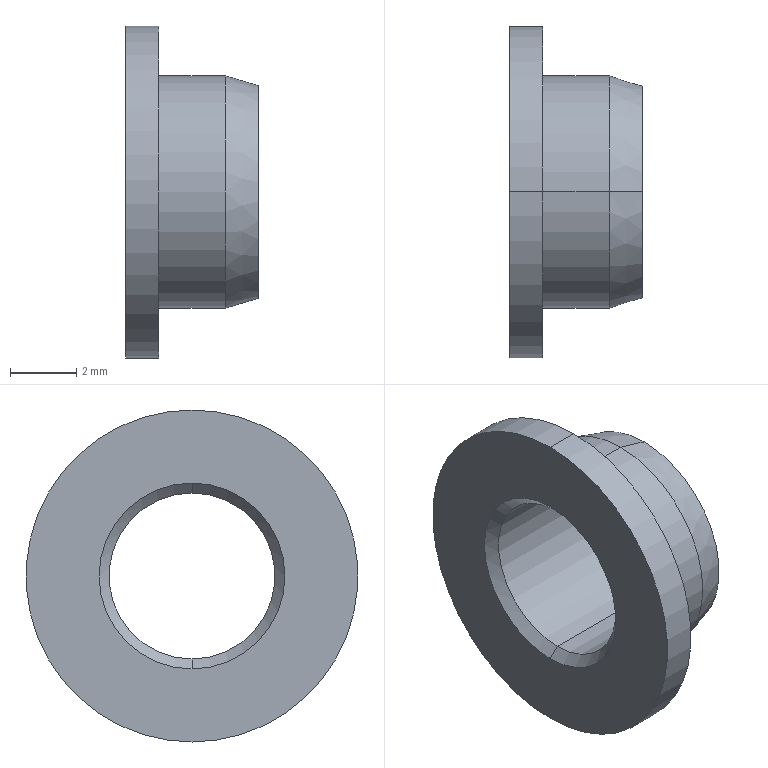Part | STEP file | 0246_010_JZF5-3 | 1 solid | 13 faces | box 4 x 10 x 10 mm | volume 111.514 mm3 | cylinder 6 | cone 4 | plane 3 | commonest cylinder face diameters 5 x2 7 x2 10 x2
STEP:
#1=CARTESIAN_POINT('',(0.,0.,0.));
#2=DIRECTION('',(0.,0.,1.));
#3=DIRECTION('',(1.,0.,0.));
#4=AXIS2_PLACEMENT_3D('',#1,#2,#3);
#5=CARTESIAN_POINT('',(0.,0.,5.));
#6=VERTEX_POINT('',#5);
#7=CARTESIAN_POINT('',(0.,0.,-5.));
#8=VERTEX_POINT('',#7);
#9=CARTESIAN_POINT('',(0.,0.,0.));
#10=DIRECTION('',(-1.,0.,0.));
#11=DIRECTION('',(0.,0.,-1.));
#12=AXIS2_PLACEMENT_3D('',#9,#10,#11);
#13=CIRCLE('',#12,5.);
#14=CARTESIAN_POINT('',(0.5,0.,0.));
#15=DIRECTION('',(1.,0.,0.));
#16=DIRECTION('',(0.,0.,-1.));
#17=AXIS2_PLACEMENT_3D('',#14,#15,#16);
#18=CYLINDRICAL_SURFACE('',#17,5.);
#19=CARTESIAN_POINT('',(6.283,-0.5));
#20=DIRECTION('',(-1.,0.));
#21=VECTOR('',#20,1.);
#22=LINE('',#19,#21);
#23=(GEOMETRIC_REPRESENTATION_CONTEXT(2)PARAMETRIC_REPRESENTATION_CONTEXT()REPRESENTATION_CONTEXT('',''));
#24=DEFINITIONAL_REPRESENTATION('',(#22),#23);
#25=PCURVE('',#18,#24);
#26=CARTESIAN_POINT('',(0.,3.9,0.));
#27=DIRECTION('',(-1.,0.,0.));
#28=DIRECTION('',(0.,0.,1.));
#29=AXIS2_PLACEMENT_3D('',#26,#27,#28);
#30=PLANE('',#29);
#31=CARTESIAN_POINT('',(0.,-3.9));
#32=DIRECTION('',(-1.,0.));
#33=AXIS2_PLACEMENT_2D('',#31,#32);
#34=CIRCLE('',#33,5.);
#35=(GEOMETRIC_REPRESENTATION_CONTEXT(2)PARAMETRIC_REPRESENTATION_CONTEXT()REPRESENTATION_CONTEXT('',''));
#36=DEFINITIONAL_REPRESENTATION('',(#34),#35);
#37=PCURVE('',#30,#36);
#38=SURFACE_CURVE('',#13,(#25,#37),.PCURVE_S1.);
#39=EDGE_CURVE('',#6,#8,#38,.T.);
#40=ORIENTED_EDGE('',*,*,#39,.F.);
#41=CARTESIAN_POINT('',(1.,0.,5.));
#42=VERTEX_POINT('',#41);
#43=CARTESIAN_POINT('',(0.5,0.,5.));
#44=DIRECTION('',(1.,0.,0.));
#45=VECTOR('',#44,1.);
#46=LINE('',#43,#45);
#47=CARTESIAN_POINT('',(3.142,0.));
#48=DIRECTION('',(0.,1.));
#49=VECTOR('',#48,1.);
#50=LINE('',#47,#49);
#51=(GEOMETRIC_REPRESENTATION_CONTEXT(2)PARAMETRIC_REPRESENTATION_CONTEXT()REPRESENTATION_CONTEXT('',''));
#52=DEFINITIONAL_REPRESENTATION('',(#50),#51);
#53=PCURVE('',#18,#52);
#54=CARTESIAN_POINT('',(0.5,0.,0.));
#55=DIRECTION('',(1.,0.,0.));
#56=DIRECTION('',(0.,0.,-1.));
#57=AXIS2_PLACEMENT_3D('',#54,#55,#56);
#58=CYLINDRICAL_SURFACE('',#57,5.);
#59=CARTESIAN_POINT('',(3.142,0.));
#60=DIRECTION('',(0.,1.));
#61=VECTOR('',#60,1.);
#62=LINE('',#59,#61);
#63=(GEOMETRIC_REPRESENTATION_CONTEXT(2)PARAMETRIC_REPRESENTATION_CONTEXT()REPRESENTATION_CONTEXT('',''));
#64=DEFINITIONAL_REPRESENTATION('',(#62),#63);
#65=PCURVE('',#58,#64);
#66=SURFACE_CURVE('',#46,(#53,#65),.PCURVE_S1.);
#67=EDGE_CURVE('',#6,#42,#66,.T.);
#68=ORIENTED_EDGE('',*,*,#67,.T.);
#69=CARTESIAN_POINT('',(1.,0.,-5.));
#70=VERTEX_POINT('',#69);
#71=CARTESIAN_POINT('',(1.,0.,0.));
#72=DIRECTION('',(-1.,0.,0.));
#73=DIRECTION('',(0.,0.,-1.));
#74=AXIS2_PLACEMENT_3D('',#71,#72,#73);
#75=CIRCLE('',#74,5.);
#76=CARTESIAN_POINT('',(6.283,0.5));
#77=DIRECTION('',(-1.,0.));
#78=VECTOR('',#77,1.);
#79=LINE('',#76,#78);
#80=(GEOMETRIC_REPRESENTATION_CONTEXT(2)PARAMETRIC_REPRESENTATION_CONTEXT()REPRESENTATION_CONTEXT('',''));
#81=DEFINITIONAL_REPRESENTATION('',(#79),#80);
#82=PCURVE('',#18,#81);
#83=CARTESIAN_POINT('',(1.,4.25,0.));
#84=DIRECTION('',(1.,0.,0.));
#85=DIRECTION('',(0.,0.,-1.));
#86=AXIS2_PLACEMENT_3D('',#83,#84,#85);
#87=PLANE('',#86);
#88=CARTESIAN_POINT('',(5.,-4.25));
#89=CARTESIAN_POINT('',(5.,-12.91));
#90=CARTESIAN_POINT('',(-2.5,-8.58));
#91=CARTESIAN_POINT('',(-10.,-4.25));
#92=CARTESIAN_POINT('',(-2.5,0.08013));
#93=CARTESIAN_POINT('',(5.,4.41));
#94=CARTESIAN_POINT('',(5.,-4.25));
#95=(BOUNDED_CURVE()B_SPLINE_CURVE(2,(#88,#89,#90,#91,#92,#93,#94),.UNSPECIFIED.,.T.,.F.)B_SPLINE_CURVE_WITH_KNOTS((1,2,2,2,2,1),(-2.094,0.,2.094,4.189,6.283,8.378),.UNSPECIFIED.)CURVE()GEOMETRIC_REPRESENTATION_ITEM()RATIONAL_B_SPLINE_CURVE((1.,0.5,1.,0.5,1.,0.5,1.))REPRESENTATION_ITEM(''));
#96=(GEOMETRIC_REPRESENTATION_CONTEXT(2)PARAMETRIC_REPRESENTATION_CONTEXT()REPRESENTATION_CONTEXT('',''));
#97=DEFINITIONAL_REPRESENTATION('',(#95),#96);
#98=PCURVE('',#87,#97);
#99=SURFACE_CURVE('',#75,(#82,#98),.PCURVE_S1.);
#100=EDGE_CURVE('',#42,#70,#99,.T.);
#101=ORIENTED_EDGE('',*,*,#100,.T.);
#102=CARTESIAN_POINT('',(0.5,0.,-5.));
#103=DIRECTION('',(1.,0.,0.));
#104=VECTOR('',#103,1.);
#105=LINE('',#102,#104);
#106=CARTESIAN_POINT('',(0.,0.));
#107=DIRECTION('',(0.,1.));
#108=VECTOR('',#107,1.);
#109=LINE('',#106,#108);
#110=(GEOMETRIC_REPRESENTATION_CONTEXT(2)PARAMETRIC_REPRESENTATION_CONTEXT()REPRESENTATION_CONTEXT('',''));
#111=DEFINITIONAL_REPRESENTATION('',(#109),#110);
#112=PCURVE('',#18,#111);
#113=CARTESIAN_POINT('',(6.283,0.));
#114=DIRECTION('',(0.,1.));
#115=VECTOR('',#114,1.);
#116=LINE('',#113,#115);
#117=(GEOMETRIC_REPRESENTATION_CONTEXT(2)PARAMETRIC_REPRESENTATION_CONTEXT()REPRESENTATION_CONTEXT('',''));
#118=DEFINITIONAL_REPRESENTATION('',(#116),#117);
#119=PCURVE('',#58,#118);
#120=SURFACE_CURVE('',#105,(#112,#119),.PCURVE_S1.);
#121=EDGE_CURVE('',#8,#70,#120,.T.);
#122=ORIENTED_EDGE('',*,*,#121,.F.);
#123=EDGE_LOOP('',(#40,#68,#101,#122));
#124=FACE_BOUND('',#123,.T.);
#125=ADVANCED_FACE('',(#124),#18,.T.);
#126=CARTESIAN_POINT('',(0.3,0.,2.5));
#127=VERTEX_POINT('',#126);
#128=CARTESIAN_POINT('',(0.,0.,2.8));
#129=VERTEX_POINT('',#128);
#130=CARTESIAN_POINT('',(0.,0.,2.8));
#131=DIRECTION('',(-0.7071,0.,0.7071));
#132=VECTOR('',#131,1.);
#133=LINE('',#130,#132);
#134=CARTESIAN_POINT('',(0.,0.,0.));
#135=DIRECTION('',(-1.,0.,0.));
#136=DIRECTION('',(0.,0.,1.));
#137=AXIS2_PLACEMENT_3D('',#134,#135,#136);
#138=CONICAL_SURFACE('',#137,2.8,0.7854);
#139=CARTESIAN_POINT('',(6.283,0.));
#140=DIRECTION('',(0.,1.));
#141=VECTOR('',#140,1.);
#142=LINE('',#139,#141);
#143=(GEOMETRIC_REPRESENTATION_CONTEXT(2)PARAMETRIC_REPRESENTATION_CONTEXT()REPRESENTATION_CONTEXT('',''));
#144=DEFINITIONAL_REPRESENTATION('',(#142),#143);
#145=PCURVE('',#138,#144);
#146=CARTESIAN_POINT('',(0.,0.,0.));
#147=DIRECTION('',(-1.,0.,0.));
#148=DIRECTION('',(0.,0.,1.));
#149=AXIS2_PLACEMENT_3D('',#146,#147,#148);
#150=CONICAL_SURFACE('',#149,2.8,0.7854);
#151=CARTESIAN_POINT('',(0.,0.));
#152=DIRECTION('',(0.,1.));
#153=VECTOR('',#152,1.);
#154=LINE('',#151,#153);
#155=(GEOMETRIC_REPRESENTATION_CONTEXT(2)PARAMETRIC_REPRESENTATION_CONTEXT()REPRESENTATION_CONTEXT('',''));
#156=DEFINITIONAL_REPRESENTATION('',(#154),#155);
#157=PCURVE('',#150,#156);
#158=SURFACE_CURVE('',#133,(#145,#157),.PCURVE_S1.);
#159=EDGE_CURVE('',#127,#129,#158,.T.);
#160=ORIENTED_EDGE('',*,*,#159,.T.);
#161=CARTESIAN_POINT('',(0.,0.,-2.8));
#162=VERTEX_POINT('',#161);
#163=CARTESIAN_POINT('',(0.,0.,0.));
#164=DIRECTION('',(1.,0.,0.));
#165=DIRECTION('',(0.,0.,1.));
#166=AXIS2_PLACEMENT_3D('',#163,#164,#165);
#167=CIRCLE('',#166,2.8);
#168=CARTESIAN_POINT('',(6.283,0.));
#169=DIRECTION('',(-1.,0.));
#170=VECTOR('',#169,1.);
#171=LINE('',#168,#170);
#172=(GEOMETRIC_REPRESENTATION_CONTEXT(2)PARAMETRIC_REPRESENTATION_CONTEXT()REPRESENTATION_CONTEXT('',''));
#173=DEFINITIONAL_REPRESENTATION('',(#171),#172);
#174=PCURVE('',#138,#173);
#175=CARTESIAN_POINT('',(2.8,-3.9));
#176=CARTESIAN_POINT('',(2.8,-8.75));
#177=CARTESIAN_POINT('',(-1.4,-6.325));
#178=CARTESIAN_POINT('',(-5.6,-3.9));
#179=CARTESIAN_POINT('',(-1.4,-1.475));
#180=CARTESIAN_POINT('',(2.8,0.9497));
#181=CARTESIAN_POINT('',(2.8,-3.9));
#182=(BOUNDED_CURVE()B_SPLINE_CURVE(2,(#175,#176,#177,#178,#179,#180,#181),.UNSPECIFIED.,.T.,.F.)B_SPLINE_CURVE_WITH_KNOTS((1,2,2,2,2,1),(-2.094,0.,2.094,4.189,6.283,8.378),.UNSPECIFIED.)CURVE()GEOMETRIC_REPRESENTATION_ITEM()RATIONAL_B_SPLINE_CURVE((1.,0.5,1.,0.5,1.,0.5,1.))REPRESENTATION_ITEM(''));
#183=(GEOMETRIC_REPRESENTATION_CONTEXT(2)PARAMETRIC_REPRESENTATION_CONTEXT()REPRESENTATION_CONTEXT('',''));
#184=DEFINITIONAL_REPRESENTATION('',(#182),#183);
#185=PCURVE('',#30,#184);
#186=SURFACE_CURVE('',#167,(#174,#185),.PCURVE_S1.);
#187=EDGE_CURVE('',#129,#162,#186,.T.);
#188=ORIENTED_EDGE('',*,*,#187,.T.);
#189=CARTESIAN_POINT('',(0.3,0.,-2.5));
#190=VERTEX_POINT('',#189);
#191=CARTESIAN_POINT('',(0.,0.,-2.8));
#192=DIRECTION('',(-0.7071,0.,-0.7071));
#193=VECTOR('',#192,1.);
#194=LINE('',#191,#193);
#195=CARTESIAN_POINT('',(3.142,0.));
#196=DIRECTION('',(0.,1.));
#197=VECTOR('',#196,1.);
#198=LINE('',#195,#197);
#199=(GEOMETRIC_REPRESENTATION_CONTEXT(2)PARAMETRIC_REPRESENTATION_CONTEXT()REPRESENTATION_CONTEXT('',''));
#200=DEFINITIONAL_REPRESENTATION('',(#198),#199);
#201=PCURVE('',#138,#200);
#202=CARTESIAN_POINT('',(3.142,0.));
#203=DIRECTION('',(0.,1.));
#204=VECTOR('',#203,1.);
#205=LINE('',#202,#204);
#206=(GEOMETRIC_REPRESENTATION_CONTEXT(2)PARAMETRIC_REPRESENTATION_CONTEXT()REPRESENTATION_CONTEXT('',''));
#207=DEFINITIONAL_REPRESENTATION('',(#205),#206);
#208=PCURVE('',#150,#207);
#209=SURFACE_CURVE('',#194,(#201,#208),.PCURVE_S1.);
#210=EDGE_CURVE('',#190,#162,#209,.T.);
#211=ORIENTED_EDGE('',*,*,#210,.F.);
#212=CARTESIAN_POINT('',(0.3,0.,0.));
#213=DIRECTION('',(-1.,0.,0.));
#214=DIRECTION('',(0.,1.,0.));
#215=AXIS2_PLACEMENT_3D('',#212,#213,#214);
#216=CIRCLE('',#215,2.5);
#217=CARTESIAN_POINT('',(1.571,-0.3));
#218=DIRECTION('',(1.,0.));
#219=VECTOR('',#218,1.);
#220=LINE('',#217,#219);
#221=(GEOMETRIC_REPRESENTATION_CONTEXT(2)PARAMETRIC_REPRESENTATION_CONTEXT()REPRESENTATION_CONTEXT('',''));
#222=DEFINITIONAL_REPRESENTATION('',(#220),#221);
#223=PCURVE('',#138,#222);
#224=CARTESIAN_POINT('',(2.15,0.,0.));
#225=DIRECTION('',(1.,0.,0.));
#226=DIRECTION('',(0.,0.,-1.));
#227=AXIS2_PLACEMENT_3D('',#224,#225,#226);
#228=CYLINDRICAL_SURFACE('',#227,2.5);
#229=CARTESIAN_POINT('',(7.854,-1.85));
#230=DIRECTION('',(-1.,0.));
#231=VECTOR('',#230,1.);
#232=LINE('',#229,#231);
#233=(GEOMETRIC_REPRESENTATION_CONTEXT(2)PARAMETRIC_REPRESENTATION_CONTEXT()REPRESENTATION_CONTEXT('',''));
#234=DEFINITIONAL_REPRESENTATION('',(#232),#233);
#235=PCURVE('',#228,#234);
#236=SURFACE_CURVE('',#216,(#223,#235),.PCURVE_S1.);
#237=EDGE_CURVE('',#190,#127,#236,.T.);
#238=ORIENTED_EDGE('',*,*,#237,.T.);
#239=EDGE_LOOP('',(#160,#188,#211,#238));
#240=FACE_BOUND('',#239,.F.);
#241=ADVANCED_FACE('',(#240),#138,.F.);
#242=CARTESIAN_POINT('',(4.,0.,-2.5));
#243=VERTEX_POINT('',#242);
#244=CARTESIAN_POINT('',(2.15,0.,-2.5));
#245=DIRECTION('',(1.,0.,0.));
#246=VECTOR('',#245,1.);
#247=LINE('',#244,#246);
#248=CARTESIAN_POINT('',(6.283,0.));
#249=DIRECTION('',(0.,1.));
#250=VECTOR('',#249,1.);
#251=LINE('',#248,#250);
#252=(GEOMETRIC_REPRESENTATION_CONTEXT(2)PARAMETRIC_REPRESENTATION_CONTEXT()REPRESENTATION_CONTEXT('',''));
#253=DEFINITIONAL_REPRESENTATION('',(#251),#252);
#254=PCURVE('',#228,#253);
#255=CARTESIAN_POINT('',(2.15,0.,0.));
#256=DIRECTION('',(1.,0.,0.));
#257=DIRECTION('',(0.,0.,-1.));
#258=AXIS2_PLACEMENT_3D('',#255,#256,#257);
#259=CYLINDRICAL_SURFACE('',#258,2.5);
#260=CARTESIAN_POINT('',(0.,0.));
#261=DIRECTION('',(0.,1.));
#262=VECTOR('',#261,1.);
#263=LINE('',#260,#262);
#264=(GEOMETRIC_REPRESENTATION_CONTEXT(2)PARAMETRIC_REPRESENTATION_CONTEXT()REPRESENTATION_CONTEXT('',''));
#265=DEFINITIONAL_REPRESENTATION('',(#263),#264);
#266=PCURVE('',#259,#265);
#267=SURFACE_CURVE('',#247,(#254,#266),.PCURVE_S1.);
#268=EDGE_CURVE('',#190,#243,#267,.T.);
#269=ORIENTED_EDGE('',*,*,#268,.T.);
#270=CARTESIAN_POINT('',(4.,0.,2.5));
#271=VERTEX_POINT('',#270);
#272=CARTESIAN_POINT('',(4.,0.,0.));
#273=DIRECTION('',(-1.,0.,0.));
#274=DIRECTION('',(0.,0.,-1.));
#275=AXIS2_PLACEMENT_3D('',#272,#273,#274);
#276=CIRCLE('',#275,2.5);
#277=CARTESIAN_POINT('',(6.283,1.85));
#278=DIRECTION('',(-1.,0.));
#279=VECTOR('',#278,1.);
#280=LINE('',#277,#279);
#281=(GEOMETRIC_REPRESENTATION_CONTEXT(2)PARAMETRIC_REPRESENTATION_CONTEXT()REPRESENTATION_CONTEXT('',''));
#282=DEFINITIONAL_REPRESENTATION('',(#280),#281);
#283=PCURVE('',#228,#282);
#284=CARTESIAN_POINT('',(4.,2.85,0.));
#285=DIRECTION('',(1.,0.,0.));
#286=DIRECTION('',(0.,0.,-1.));
#287=AXIS2_PLACEMENT_3D('',#284,#285,#286);
#288=PLANE('',#287);
#289=CARTESIAN_POINT('',(2.5,-2.85));
#290=CARTESIAN_POINT('',(2.5,-7.18));
#291=CARTESIAN_POINT('',(-1.25,-5.015));
#292=CARTESIAN_POINT('',(-5.,-2.85));
#293=CARTESIAN_POINT('',(-1.25,-0.6849));
#294=CARTESIAN_POINT('',(2.5,1.48));
#295=CARTESIAN_POINT('',(2.5,-2.85));
#296=(BOUNDED_CURVE()B_SPLINE_CURVE(2,(#289,#290,#291,#292,#293,#294,#295),.UNSPECIFIED.,.T.,.F.)B_SPLINE_CURVE_WITH_KNOTS((1,2,2,2,2,1),(-2.094,0.,2.094,4.189,6.283,8.378),.UNSPECIFIED.)CURVE()GEOMETRIC_REPRESENTATION_ITEM()RATIONAL_B_SPLINE_CURVE((1.,0.5,1.,0.5,1.,0.5,1.))REPRESENTATION_ITEM(''));
#297=(GEOMETRIC_REPRESENTATION_CONTEXT(2)PARAMETRIC_REPRESENTATION_CONTEXT()REPRESENTATION_CONTEXT('',''));
#298=DEFINITIONAL_REPRESENTATION('',(#296),#297);
#299=PCURVE('',#288,#298);
#300=SURFACE_CURVE('',#276,(#283,#299),.PCURVE_S1.);
#301=EDGE_CURVE('',#243,#271,#300,.T.);
#302=ORIENTED_EDGE('',*,*,#301,.T.);
#303=CARTESIAN_POINT('',(2.15,0.,2.5));
#304=DIRECTION('',(1.,0.,0.));
#305=VECTOR('',#304,1.);
#306=LINE('',#303,#305);
#307=CARTESIAN_POINT('',(3.142,0.));
#308=DIRECTION('',(0.,1.));
#309=VECTOR('',#308,1.);
#310=LINE('',#307,#309);
#311=(GEOMETRIC_REPRESENTATION_CONTEXT(2)PARAMETRIC_REPRESENTATION_CONTEXT()REPRESENTATION_CONTEXT('',''));
#312=DEFINITIONAL_REPRESENTATION('',(#310),#311);
#313=PCURVE('',#228,#312);
#314=CARTESIAN_POINT('',(3.142,0.));
#315=DIRECTION('',(0.,1.));
#316=VECTOR('',#315,1.);
#317=LINE('',#314,#316);
#318=(GEOMETRIC_REPRESENTATION_CONTEXT(2)PARAMETRIC_REPRESENTATION_CONTEXT()REPRESENTATION_CONTEXT('',''));
#319=DEFINITIONAL_REPRESENTATION('',(#317),#318);
#320=PCURVE('',#259,#319);
#321=SURFACE_CURVE('',#306,(#313,#320),.PCURVE_S1.);
#322=EDGE_CURVE('',#127,#271,#321,.T.);
#323=ORIENTED_EDGE('',*,*,#322,.F.);
#324=ORIENTED_EDGE('',*,*,#237,.F.);
#325=EDGE_LOOP('',(#269,#302,#323,#324));
#326=FACE_BOUND('',#325,.F.);
#327=ADVANCED_FACE('',(#326),#228,.F.);
#328=CARTESIAN_POINT('',(1.,0.,3.5));
#329=VERTEX_POINT('',#328);
#330=CARTESIAN_POINT('',(1.,0.,-3.5));
#331=VERTEX_POINT('',#330);
#332=CARTESIAN_POINT('',(1.,0.,0.));
#333=DIRECTION('',(-1.,0.,0.));
#334=DIRECTION('',(0.,0.,-1.));
#335=AXIS2_PLACEMENT_3D('',#332,#333,#334);
#336=CIRCLE('',#335,3.5);
#337=CARTESIAN_POINT('',(2.,0.,0.));
#338=DIRECTION('',(1.,0.,0.));
#339=DIRECTION('',(0.,0.,-1.));
#340=AXIS2_PLACEMENT_3D('',#337,#338,#339);
#341=CYLINDRICAL_SURFACE('',#340,3.5);
#342=CARTESIAN_POINT('',(6.283,-1.));
#343=DIRECTION('',(-1.,0.));
#344=VECTOR('',#343,1.);
#345=LINE('',#342,#344);
#346=(GEOMETRIC_REPRESENTATION_CONTEXT(2)PARAMETRIC_REPRESENTATION_CONTEXT()REPRESENTATION_CONTEXT('',''));
#347=DEFINITIONAL_REPRESENTATION('',(#345),#346);
#348=PCURVE('',#341,#347);
#349=CARTESIAN_POINT('',(3.5,-4.25));
#350=CARTESIAN_POINT('',(3.5,-10.312));
#351=CARTESIAN_POINT('',(-1.75,-7.281));
#352=CARTESIAN_POINT('',(-7.,-4.25));
#353=CARTESIAN_POINT('',(-1.75,-1.219));
#354=CARTESIAN_POINT('',(3.5,1.812));
#355=CARTESIAN_POINT('',(3.5,-4.25));
#356=(BOUNDED_CURVE()B_SPLINE_CURVE(2,(#349,#350,#351,#352,#353,#354,#355),.UNSPECIFIED.,.T.,.F.)B_SPLINE_CURVE_WITH_KNOTS((1,2,2,2,2,1),(-2.094,0.,2.094,4.189,6.283,8.378),.UNSPECIFIED.)CURVE()GEOMETRIC_REPRESENTATION_ITEM()RATIONAL_B_SPLINE_CURVE((1.,0.5,1.,0.5,1.,0.5,1.))REPRESENTATION_ITEM(''));
#357=(GEOMETRIC_REPRESENTATION_CONTEXT(2)PARAMETRIC_REPRESENTATION_CONTEXT()REPRESENTATION_CONTEXT('',''));
#358=DEFINITIONAL_REPRESENTATION('',(#356),#357);
#359=PCURVE('',#87,#358);
#360=SURFACE_CURVE('',#336,(#348,#359),.PCURVE_S1.);
#361=EDGE_CURVE('',#329,#331,#360,.T.);
#362=ORIENTED_EDGE('',*,*,#361,.F.);
#363=CARTESIAN_POINT('',(3.,0.,3.5));
#364=VERTEX_POINT('',#363);
#365=CARTESIAN_POINT('',(2.,0.,3.5));
#366=DIRECTION('',(1.,0.,0.));
#367=VECTOR('',#366,1.);
#368=LINE('',#365,#367);
#369=CARTESIAN_POINT('',(3.142,0.));
#370=DIRECTION('',(0.,1.));
#371=VECTOR('',#370,1.);
#372=LINE('',#369,#371);
#373=(GEOMETRIC_REPRESENTATION_CONTEXT(2)PARAMETRIC_REPRESENTATION_CONTEXT()REPRESENTATION_CONTEXT('',''));
#374=DEFINITIONAL_REPRESENTATION('',(#372),#373);
#375=PCURVE('',#341,#374);
#376=CARTESIAN_POINT('',(2.,0.,0.));
#377=DIRECTION('',(1.,0.,0.));
#378=DIRECTION('',(0.,0.,-1.));
#379=AXIS2_PLACEMENT_3D('',#376,#377,#378);
#380=CYLINDRICAL_SURFACE('',#379,3.5);
#381=CARTESIAN_POINT('',(3.142,0.));
#382=DIRECTION('',(0.,1.));
#383=VECTOR('',#382,1.);
#384=LINE('',#381,#383);
#385=(GEOMETRIC_REPRESENTATION_CONTEXT(2)PARAMETRIC_REPRESENTATION_CONTEXT()REPRESENTATION_CONTEXT('',''));
#386=DEFINITIONAL_REPRESENTATION('',(#384),#385);
#387=PCURVE('',#380,#386);
#388=SURFACE_CURVE('',#368,(#375,#387),.PCURVE_S1.);
#389=EDGE_CURVE('',#329,#364,#388,.T.);
#390=ORIENTED_EDGE('',*,*,#389,.T.);
#391=CARTESIAN_POINT('',(3.,0.,-3.5));
#392=VERTEX_POINT('',#391);
#393=CARTESIAN_POINT('',(3.,0.,0.));
#394=DIRECTION('',(-1.,0.,0.));
#395=DIRECTION('',(0.,0.,-1.));
#396=AXIS2_PLACEMENT_3D('',#393,#394,#395);
#397=CIRCLE('',#396,3.5);
#398=CARTESIAN_POINT('',(6.283,1.));
#399=DIRECTION('',(-1.,0.));
#400=VECTOR('',#399,1.);
#401=LINE('',#398,#400);
#402=(GEOMETRIC_REPRESENTATION_CONTEXT(2)PARAMETRIC_REPRESENTATION_CONTEXT()REPRESENTATION_CONTEXT('',''));
#403=DEFINITIONAL_REPRESENTATION('',(#401),#402);
#404=PCURVE('',#341,#403);
#405=CARTESIAN_POINT('',(3.,0.,0.));
#406=DIRECTION('',(-1.,0.,0.));
#407=DIRECTION('',(0.,0.,1.));
#408=AXIS2_PLACEMENT_3D('',#405,#406,#407);
#409=CONICAL_SURFACE('',#408,3.5,0.2915);
#410=CARTESIAN_POINT('',(-3.142,0.));
#411=DIRECTION('',(1.,0.));
#412=VECTOR('',#411,1.);
#413=LINE('',#410,#412);
#414=(GEOMETRIC_REPRESENTATION_CONTEXT(2)PARAMETRIC_REPRESENTATION_CONTEXT()REPRESENTATION_CONTEXT('',''));
#415=DEFINITIONAL_REPRESENTATION('',(#413),#414);
#416=PCURVE('',#409,#415);
#417=SURFACE_CURVE('',#397,(#404,#416),.PCURVE_S1.);
#418=EDGE_CURVE('',#364,#392,#417,.T.);
#419=ORIENTED_EDGE('',*,*,#418,.T.);
#420=CARTESIAN_POINT('',(2.,0.,-3.5));
#421=DIRECTION('',(1.,0.,0.));
#422=VECTOR('',#421,1.);
#423=LINE('',#420,#422);
#424=CARTESIAN_POINT('',(0.,0.));
#425=DIRECTION('',(0.,1.));
#426=VECTOR('',#425,1.);
#427=LINE('',#424,#426);
#428=(GEOMETRIC_REPRESENTATION_CONTEXT(2)PARAMETRIC_REPRESENTATION_CONTEXT()REPRESENTATION_CONTEXT('',''));
#429=DEFINITIONAL_REPRESENTATION('',(#427),#428);
#430=PCURVE('',#341,#429);
#431=CARTESIAN_POINT('',(6.283,0.));
#432=DIRECTION('',(0.,1.));
#433=VECTOR('',#432,1.);
#434=LINE('',#431,#433);
#435=(GEOMETRIC_REPRESENTATION_CONTEXT(2)PARAMETRIC_REPRESENTATION_CONTEXT()REPRESENTATION_CONTEXT('',''));
#436=DEFINITIONAL_REPRESENTATION('',(#434),#435);
#437=PCURVE('',#380,#436);
#438=SURFACE_CURVE('',#423,(#430,#437),.PCURVE_S1.);
#439=EDGE_CURVE('',#331,#392,#438,.T.);
#440=ORIENTED_EDGE('',*,*,#439,.F.);
#441=EDGE_LOOP('',(#362,#390,#419,#440));
#442=FACE_BOUND('',#441,.T.);
#443=ADVANCED_FACE('',(#442),#341,.T.);
#444=CARTESIAN_POINT('',(4.,0.,-3.2));
#445=VERTEX_POINT('',#444);
#446=CARTESIAN_POINT('',(4.,0.,3.2));
#447=VERTEX_POINT('',#446);
#448=CARTESIAN_POINT('',(4.,0.,0.));
#449=DIRECTION('',(1.,0.,0.));
#450=DIRECTION('',(0.,0.,1.));
#451=AXIS2_PLACEMENT_3D('',#448,#449,#450);
#452=CIRCLE('',#451,3.2);
#453=CARTESIAN_POINT('',(6.283,-1.));
#454=DIRECTION('',(-1.,0.));
#455=VECTOR('',#454,1.);
#456=LINE('',#453,#455);
#457=(GEOMETRIC_REPRESENTATION_CONTEXT(2)PARAMETRIC_REPRESENTATION_CONTEXT()REPRESENTATION_CONTEXT('',''));
#458=DEFINITIONAL_REPRESENTATION('',(#456),#457);
#459=PCURVE('',#409,#458);
#460=CARTESIAN_POINT('',(0.,-2.85));
#461=DIRECTION('',(-1.,0.));
#462=AXIS2_PLACEMENT_2D('',#460,#461);
#463=CIRCLE('',#462,3.2);
#464=(GEOMETRIC_REPRESENTATION_CONTEXT(2)PARAMETRIC_REPRESENTATION_CONTEXT()REPRESENTATION_CONTEXT('',''));
#465=DEFINITIONAL_REPRESENTATION('',(#463),#464);
#466=PCURVE('',#288,#465);
#467=SURFACE_CURVE('',#452,(#459,#466),.PCURVE_S1.);
#468=EDGE_CURVE('',#445,#447,#467,.T.);
#469=ORIENTED_EDGE('',*,*,#468,.F.);
#470=CARTESIAN_POINT('',(3.,0.,-3.5));
#471=DIRECTION('',(-0.9578,0.,-0.2873));
#472=VECTOR('',#471,1.);
#473=LINE('',#470,#472);
#474=CARTESIAN_POINT('',(3.142,0.));
#475=DIRECTION('',(0.,1.));
#476=VECTOR('',#475,1.);
#477=LINE('',#474,#476);
#478=(GEOMETRIC_REPRESENTATION_CONTEXT(2)PARAMETRIC_REPRESENTATION_CONTEXT()REPRESENTATION_CONTEXT('',''));
#479=DEFINITIONAL_REPRESENTATION('',(#477),#478);
#480=PCURVE('',#409,#479);
#481=CARTESIAN_POINT('',(3.,0.,0.));
#482=DIRECTION('',(-1.,0.,0.));
#483=DIRECTION('',(0.,0.,1.));
#484=AXIS2_PLACEMENT_3D('',#481,#482,#483);
#485=CONICAL_SURFACE('',#484,3.5,0.2915);
#486=CARTESIAN_POINT('',(3.142,0.));
#487=DIRECTION('',(0.,1.));
#488=VECTOR('',#487,1.);
#489=LINE('',#486,#488);
#490=(GEOMETRIC_REPRESENTATION_CONTEXT(2)PARAMETRIC_REPRESENTATION_CONTEXT()REPRESENTATION_CONTEXT('',''));
#491=DEFINITIONAL_REPRESENTATION('',(#489),#490);
#492=PCURVE('',#485,#491);
#493=SURFACE_CURVE('',#473,(#480,#492),.PCURVE_S1.);
#494=EDGE_CURVE('',#445,#392,#493,.T.);
#495=ORIENTED_EDGE('',*,*,#494,.T.);
#496=ORIENTED_EDGE('',*,*,#418,.F.);
#497=CARTESIAN_POINT('',(3.,0.,3.5));
#498=DIRECTION('',(-0.9578,0.,0.2873));
#499=VECTOR('',#498,1.);
#500=LINE('',#497,#499);
#501=CARTESIAN_POINT('',(0.,0.));
#502=DIRECTION('',(0.,1.));
#503=VECTOR('',#502,1.);
#504=LINE('',#501,#503);
#505=(GEOMETRIC_REPRESENTATION_CONTEXT(2)PARAMETRIC_REPRESENTATION_CONTEXT()REPRESENTATION_CONTEXT('',''));
#506=DEFINITIONAL_REPRESENTATION('',(#504),#505);
#507=PCURVE('',#409,#506);
#508=CARTESIAN_POINT('',(6.283,0.));
#509=DIRECTION('',(0.,1.));
#510=VECTOR('',#509,1.);
#511=LINE('',#508,#510);
#512=(GEOMETRIC_REPRESENTATION_CONTEXT(2)PARAMETRIC_REPRESENTATION_CONTEXT()REPRESENTATION_CONTEXT('',''));
#513=DEFINITIONAL_REPRESENTATION('',(#511),#512);
#514=PCURVE('',#485,#513);
#515=SURFACE_CURVE('',#500,(#507,#514),.PCURVE_S1.);
#516=EDGE_CURVE('',#447,#364,#515,.T.);
#517=ORIENTED_EDGE('',*,*,#516,.F.);
#518=EDGE_LOOP('',(#469,#495,#496,#517));
#519=FACE_BOUND('',#518,.T.);
#520=ADVANCED_FACE('',(#519),#409,.T.);
#521=CARTESIAN_POINT('',(0.,0.,0.));
#522=DIRECTION('',(-1.,0.,0.));
#523=DIRECTION('',(0.,0.,-1.));
#524=AXIS2_PLACEMENT_3D('',#521,#522,#523);
#525=CIRCLE('',#524,5.);
#526=CARTESIAN_POINT('',(0.,-3.9));
#527=DIRECTION('',(-1.,0.));
#528=AXIS2_PLACEMENT_2D('',#526,#527);
#529=CIRCLE('',#528,5.);
#530=(GEOMETRIC_REPRESENTATION_CONTEXT(2)PARAMETRIC_REPRESENTATION_CONTEXT()REPRESENTATION_CONTEXT('',''));
#531=DEFINITIONAL_REPRESENTATION('',(#529),#530);
#532=PCURVE('',#30,#531);
#533=CARTESIAN_POINT('',(6.283,-0.5));
#534=DIRECTION('',(-1.,0.));
#535=VECTOR('',#534,1.);
#536=LINE('',#533,#535);
#537=(GEOMETRIC_REPRESENTATION_CONTEXT(2)PARAMETRIC_REPRESENTATION_CONTEXT()REPRESENTATION_CONTEXT('',''));
#538=DEFINITIONAL_REPRESENTATION('',(#536),#537);
#539=PCURVE('',#58,#538);
#540=SURFACE_CURVE('',#525,(#532,#539),.PCURVE_S1.);
#541=EDGE_CURVE('',#8,#6,#540,.T.);
#542=ORIENTED_EDGE('',*,*,#541,.T.);
#543=ORIENTED_EDGE('',*,*,#39,.T.);
#544=EDGE_LOOP('',(#542,#543));
#545=FACE_BOUND('',#544,.T.);
#546=ORIENTED_EDGE('',*,*,#187,.T.);
#547=CARTESIAN_POINT('',(0.,0.,0.));
#548=DIRECTION('',(1.,0.,0.));
#549=DIRECTION('',(0.,0.,1.));
#550=AXIS2_PLACEMENT_3D('',#547,#548,#549);
#551=CIRCLE('',#550,2.8);
#552=CARTESIAN_POINT('',(2.8,-3.9));
#553=CARTESIAN_POINT('',(2.8,-8.75));
#554=CARTESIAN_POINT('',(-1.4,-6.325));
#555=CARTESIAN_POINT('',(-5.6,-3.9));
#556=CARTESIAN_POINT('',(-1.4,-1.475));
#557=CARTESIAN_POINT('',(2.8,0.9497));
#558=CARTESIAN_POINT('',(2.8,-3.9));
#559=(BOUNDED_CURVE()B_SPLINE_CURVE(2,(#552,#553,#554,#555,#556,#557,#558),.UNSPECIFIED.,.T.,.F.)B_SPLINE_CURVE_WITH_KNOTS((1,2,2,2,2,1),(-2.094,0.,2.094,4.189,6.283,8.378),.UNSPECIFIED.)CURVE()GEOMETRIC_REPRESENTATION_ITEM()RATIONAL_B_SPLINE_CURVE((1.,0.5,1.,0.5,1.,0.5,1.))REPRESENTATION_ITEM(''));
#560=(GEOMETRIC_REPRESENTATION_CONTEXT(2)PARAMETRIC_REPRESENTATION_CONTEXT()REPRESENTATION_CONTEXT('',''));
#561=DEFINITIONAL_REPRESENTATION('',(#559),#560);
#562=PCURVE('',#30,#561);
#563=CARTESIAN_POINT('',(6.283,0.));
#564=DIRECTION('',(-1.,0.));
#565=VECTOR('',#564,1.);
#566=LINE('',#563,#565);
#567=(GEOMETRIC_REPRESENTATION_CONTEXT(2)PARAMETRIC_REPRESENTATION_CONTEXT()REPRESENTATION_CONTEXT('',''));
#568=DEFINITIONAL_REPRESENTATION('',(#566),#567);
#569=PCURVE('',#150,#568);
#570=SURFACE_CURVE('',#551,(#562,#569),.PCURVE_S1.);
#571=EDGE_CURVE('',#162,#129,#570,.T.);
#572=ORIENTED_EDGE('',*,*,#571,.T.);
#573=EDGE_LOOP('',(#546,#572));
#574=FACE_BOUND('',#573,.T.);
#575=ADVANCED_FACE('',(#545,#574),#30,.T.);
#576=ORIENTED_EDGE('',*,*,#67,.F.);
#577=ORIENTED_EDGE('',*,*,#541,.F.);
#578=ORIENTED_EDGE('',*,*,#121,.T.);
#579=CARTESIAN_POINT('',(1.,0.,0.));
#580=DIRECTION('',(-1.,0.,0.));
#581=DIRECTION('',(0.,0.,-1.));
#582=AXIS2_PLACEMENT_3D('',#579,#580,#581);
#583=CIRCLE('',#582,5.);
#584=CARTESIAN_POINT('',(6.283,0.5));
#585=DIRECTION('',(-1.,0.));
#586=VECTOR('',#585,1.);
#587=LINE('',#584,#586);
#588=(GEOMETRIC_REPRESENTATION_CONTEXT(2)PARAMETRIC_REPRESENTATION_CONTEXT()REPRESENTATION_CONTEXT('',''));
#589=DEFINITIONAL_REPRESENTATION('',(#587),#588);
#590=PCURVE('',#58,#589);
#591=CARTESIAN_POINT('',(5.,-4.25));
#592=CARTESIAN_POINT('',(5.,-12.91));
#593=CARTESIAN_POINT('',(-2.5,-8.58));
#594=CARTESIAN_POINT('',(-10.,-4.25));
#595=CARTESIAN_POINT('',(-2.5,0.08013));
#596=CARTESIAN_POINT('',(5.,4.41));
#597=CARTESIAN_POINT('',(5.,-4.25));
#598=(BOUNDED_CURVE()B_SPLINE_CURVE(2,(#591,#592,#593,#594,#595,#596,#597),.UNSPECIFIED.,.T.,.F.)B_SPLINE_CURVE_WITH_KNOTS((1,2,2,2,2,1),(-2.094,0.,2.094,4.189,6.283,8.378),.UNSPECIFIED.)CURVE()GEOMETRIC_REPRESENTATION_ITEM()RATIONAL_B_SPLINE_CURVE((1.,0.5,1.,0.5,1.,0.5,1.))REPRESENTATION_ITEM(''));
#599=(GEOMETRIC_REPRESENTATION_CONTEXT(2)PARAMETRIC_REPRESENTATION_CONTEXT()REPRESENTATION_CONTEXT('',''));
#600=DEFINITIONAL_REPRESENTATION('',(#598),#599);
#601=PCURVE('',#87,#600);
#602=SURFACE_CURVE('',#583,(#590,#601),.PCURVE_S1.);
#603=EDGE_CURVE('',#70,#42,#602,.T.);
#604=ORIENTED_EDGE('',*,*,#603,.T.);
#605=EDGE_LOOP('',(#576,#577,#578,#604));
#606=FACE_BOUND('',#605,.T.);
#607=ADVANCED_FACE('',(#606),#58,.T.);
#608=ORIENTED_EDGE('',*,*,#571,.T.);
#609=ORIENTED_EDGE('',*,*,#159,.F.);
#610=CARTESIAN_POINT('',(0.3,0.,0.));
#611=DIRECTION('',(-1.,0.,0.));
#612=DIRECTION('',(0.,1.,0.));
#613=AXIS2_PLACEMENT_3D('',#610,#611,#612);
#614=CIRCLE('',#613,2.5);
#615=CARTESIAN_POINT('',(-4.712,-0.3));
#616=DIRECTION('',(1.,0.));
#617=VECTOR('',#616,1.);
#618=LINE('',#615,#617);
#619=(GEOMETRIC_REPRESENTATION_CONTEXT(2)PARAMETRIC_REPRESENTATION_CONTEXT()REPRESENTATION_CONTEXT('',''));
#620=DEFINITIONAL_REPRESENTATION('',(#618),#619);
#621=PCURVE('',#150,#620);
#622=CARTESIAN_POINT('',(7.854,-1.85));
#623=DIRECTION('',(-1.,0.));
#624=VECTOR('',#623,1.);
#625=LINE('',#622,#624);
#626=(GEOMETRIC_REPRESENTATION_CONTEXT(2)PARAMETRIC_REPRESENTATION_CONTEXT()REPRESENTATION_CONTEXT('',''));
#627=DEFINITIONAL_REPRESENTATION('',(#625),#626);
#628=PCURVE('',#259,#627);
#629=SURFACE_CURVE('',#614,(#621,#628),.PCURVE_S1.);
#630=EDGE_CURVE('',#127,#190,#629,.T.);
#631=ORIENTED_EDGE('',*,*,#630,.T.);
#632=ORIENTED_EDGE('',*,*,#210,.T.);
#633=EDGE_LOOP('',(#608,#609,#631,#632));
#634=FACE_BOUND('',#633,.F.);
#635=ADVANCED_FACE('',(#634),#150,.F.);
#636=CARTESIAN_POINT('',(1.,0.,0.));
#637=DIRECTION('',(-1.,0.,0.));
#638=DIRECTION('',(0.,0.,-1.));
#639=AXIS2_PLACEMENT_3D('',#636,#637,#638);
#640=CIRCLE('',#639,3.5);
#641=CARTESIAN_POINT('',(3.5,-4.25));
#642=CARTESIAN_POINT('',(3.5,-10.312));
#643=CARTESIAN_POINT('',(-1.75,-7.281));
#644=CARTESIAN_POINT('',(-7.,-4.25));
#645=CARTESIAN_POINT('',(-1.75,-1.219));
#646=CARTESIAN_POINT('',(3.5,1.812));
#647=CARTESIAN_POINT('',(3.5,-4.25));
#648=(BOUNDED_CURVE()B_SPLINE_CURVE(2,(#641,#642,#643,#644,#645,#646,#647),.UNSPECIFIED.,.T.,.F.)B_SPLINE_CURVE_WITH_KNOTS((1,2,2,2,2,1),(-2.094,0.,2.094,4.189,6.283,8.378),.UNSPECIFIED.)CURVE()GEOMETRIC_REPRESENTATION_ITEM()RATIONAL_B_SPLINE_CURVE((1.,0.5,1.,0.5,1.,0.5,1.))REPRESENTATION_ITEM(''));
#649=(GEOMETRIC_REPRESENTATION_CONTEXT(2)PARAMETRIC_REPRESENTATION_CONTEXT()REPRESENTATION_CONTEXT('',''));
#650=DEFINITIONAL_REPRESENTATION('',(#648),#649);
#651=PCURVE('',#87,#650);
#652=CARTESIAN_POINT('',(6.283,-1.));
#653=DIRECTION('',(-1.,0.));
#654=VECTOR('',#653,1.);
#655=LINE('',#652,#654);
#656=(GEOMETRIC_REPRESENTATION_CONTEXT(2)PARAMETRIC_REPRESENTATION_CONTEXT()REPRESENTATION_CONTEXT('',''));
#657=DEFINITIONAL_REPRESENTATION('',(#655),#656);
#658=PCURVE('',#380,#657);
#659=SURFACE_CURVE('',#640,(#651,#658),.PCURVE_S1.);
#660=EDGE_CURVE('',#331,#329,#659,.T.);
#661=ORIENTED_EDGE('',*,*,#660,.T.);
#662=ORIENTED_EDGE('',*,*,#361,.T.);
#663=EDGE_LOOP('',(#661,#662));
#664=FACE_BOUND('',#663,.T.);
#665=ORIENTED_EDGE('',*,*,#603,.F.);
#666=ORIENTED_EDGE('',*,*,#100,.F.);
#667=EDGE_LOOP('',(#665,#666));
#668=FACE_BOUND('',#667,.T.);
#669=ADVANCED_FACE('',(#664,#668),#87,.T.);
#670=CARTESIAN_POINT('',(4.,0.,0.));
#671=DIRECTION('',(-1.,0.,0.));
#672=DIRECTION('',(0.,0.,-1.));
#673=AXIS2_PLACEMENT_3D('',#670,#671,#672);
#674=CIRCLE('',#673,2.5);
#675=CARTESIAN_POINT('',(6.283,1.85));
#676=DIRECTION('',(-1.,0.));
#677=VECTOR('',#676,1.);
#678=LINE('',#675,#677);
#679=(GEOMETRIC_REPRESENTATION_CONTEXT(2)PARAMETRIC_REPRESENTATION_CONTEXT()REPRESENTATION_CONTEXT('',''));
#680=DEFINITIONAL_REPRESENTATION('',(#678),#679);
#681=PCURVE('',#259,#680);
#682=CARTESIAN_POINT('',(2.5,-2.85));
#683=CARTESIAN_POINT('',(2.5,-7.18));
#684=CARTESIAN_POINT('',(-1.25,-5.015));
#685=CARTESIAN_POINT('',(-5.,-2.85));
#686=CARTESIAN_POINT('',(-1.25,-0.6849));
#687=CARTESIAN_POINT('',(2.5,1.48));
#688=CARTESIAN_POINT('',(2.5,-2.85));
#689=(BOUNDED_CURVE()B_SPLINE_CURVE(2,(#682,#683,#684,#685,#686,#687,#688),.UNSPECIFIED.,.T.,.F.)B_SPLINE_CURVE_WITH_KNOTS((1,2,2,2,2,1),(-2.094,0.,2.094,4.189,6.283,8.378),.UNSPECIFIED.)CURVE()GEOMETRIC_REPRESENTATION_ITEM()RATIONAL_B_SPLINE_CURVE((1.,0.5,1.,0.5,1.,0.5,1.))REPRESENTATION_ITEM(''));
#690=(GEOMETRIC_REPRESENTATION_CONTEXT(2)PARAMETRIC_REPRESENTATION_CONTEXT()REPRESENTATION_CONTEXT('',''));
#691=DEFINITIONAL_REPRESENTATION('',(#689),#690);
#692=PCURVE('',#288,#691);
#693=SURFACE_CURVE('',#674,(#681,#692),.PCURVE_S1.);
#694=EDGE_CURVE('',#271,#243,#693,.T.);
#695=ORIENTED_EDGE('',*,*,#694,.T.);
#696=ORIENTED_EDGE('',*,*,#268,.F.);
#697=ORIENTED_EDGE('',*,*,#630,.F.);
#698=ORIENTED_EDGE('',*,*,#322,.T.);
#699=EDGE_LOOP('',(#695,#696,#697,#698));
#700=FACE_BOUND('',#699,.F.);
#701=ADVANCED_FACE('',(#700),#259,.F.);
#702=ORIENTED_EDGE('',*,*,#389,.F.);
#703=ORIENTED_EDGE('',*,*,#660,.F.);
#704=ORIENTED_EDGE('',*,*,#439,.T.);
#705=CARTESIAN_POINT('',(3.,0.,0.));
#706=DIRECTION('',(-1.,0.,0.));
#707=DIRECTION('',(0.,0.,-1.));
#708=AXIS2_PLACEMENT_3D('',#705,#706,#707);
#709=CIRCLE('',#708,3.5);
#710=CARTESIAN_POINT('',(6.283,1.));
#711=DIRECTION('',(-1.,0.));
#712=VECTOR('',#711,1.);
#713=LINE('',#710,#712);
#714=(GEOMETRIC_REPRESENTATION_CONTEXT(2)PARAMETRIC_REPRESENTATION_CONTEXT()REPRESENTATION_CONTEXT('',''));
#715=DEFINITIONAL_REPRESENTATION('',(#713),#714);
#716=PCURVE('',#380,#715);
#717=CARTESIAN_POINT('',(3.142,0.));
#718=DIRECTION('',(1.,0.));
#719=VECTOR('',#718,1.);
#720=LINE('',#717,#719);
#721=(GEOMETRIC_REPRESENTATION_CONTEXT(2)PARAMETRIC_REPRESENTATION_CONTEXT()REPRESENTATION_CONTEXT('',''));
#722=DEFINITIONAL_REPRESENTATION('',(#720),#721);
#723=PCURVE('',#485,#722);
#724=SURFACE_CURVE('',#709,(#716,#723),.PCURVE_S1.);
#725=EDGE_CURVE('',#392,#364,#724,.T.);
#726=ORIENTED_EDGE('',*,*,#725,.T.);
#727=EDGE_LOOP('',(#702,#703,#704,#726));
#728=FACE_BOUND('',#727,.T.);
#729=ADVANCED_FACE('',(#728),#380,.T.);
#730=ORIENTED_EDGE('',*,*,#301,.T.);
#731=ORIENTED_EDGE('',*,*,#694,.T.);
#732=EDGE_LOOP('',(#730,#731));
#733=FACE_BOUND('',#732,.T.);
#734=CARTESIAN_POINT('',(4.,0.,0.));
#735=DIRECTION('',(1.,0.,0.));
#736=DIRECTION('',(0.,0.,1.));
#737=AXIS2_PLACEMENT_3D('',#734,#735,#736);
#738=CIRCLE('',#737,3.2);
#739=CARTESIAN_POINT('',(0.,-2.85));
#740=DIRECTION('',(-1.,0.));
#741=AXIS2_PLACEMENT_2D('',#739,#740);
#742=CIRCLE('',#741,3.2);
#743=(GEOMETRIC_REPRESENTATION_CONTEXT(2)PARAMETRIC_REPRESENTATION_CONTEXT()REPRESENTATION_CONTEXT('',''));
#744=DEFINITIONAL_REPRESENTATION('',(#742),#743);
#745=PCURVE('',#288,#744);
#746=CARTESIAN_POINT('',(6.283,-1.));
#747=DIRECTION('',(-1.,0.));
#748=VECTOR('',#747,1.);
#749=LINE('',#746,#748);
#750=(GEOMETRIC_REPRESENTATION_CONTEXT(2)PARAMETRIC_REPRESENTATION_CONTEXT()REPRESENTATION_CONTEXT('',''));
#751=DEFINITIONAL_REPRESENTATION('',(#749),#750);
#752=PCURVE('',#485,#751);
#753=SURFACE_CURVE('',#738,(#745,#752),.PCURVE_S1.);
#754=EDGE_CURVE('',#447,#445,#753,.T.);
#755=ORIENTED_EDGE('',*,*,#754,.T.);
#756=ORIENTED_EDGE('',*,*,#468,.T.);
#757=EDGE_LOOP('',(#755,#756));
#758=FACE_BOUND('',#757,.T.);
#759=ADVANCED_FACE('',(#733,#758),#288,.T.);
#760=ORIENTED_EDGE('',*,*,#494,.F.);
#761=ORIENTED_EDGE('',*,*,#754,.F.);
#762=ORIENTED_EDGE('',*,*,#516,.T.);
#763=ORIENTED_EDGE('',*,*,#725,.F.);
#764=EDGE_LOOP('',(#760,#761,#762,#763));
#765=FACE_BOUND('',#764,.T.);
#766=ADVANCED_FACE('',(#765),#485,.T.);
#767=CLOSED_SHELL('',(#125,#241,#327,#443,#520,#575,#607,#635,#669,#701,#729,#759,#766));
#768=MANIFOLD_SOLID_BREP('',#767);
#769=(LENGTH_UNIT()NAMED_UNIT(*)SI_UNIT(.MILLI.,.METRE.));
#770=UNCERTAINTY_MEASURE_WITH_UNIT(LENGTH_MEASURE(0.0000001),#769,'','');
#771=(NAMED_UNIT(*)PLANE_ANGLE_UNIT()SI_UNIT($,.RADIAN.));
#772=(NAMED_UNIT(*)SI_UNIT($,.STERADIAN.)SOLID_ANGLE_UNIT());
#773=(GEOMETRIC_REPRESENTATION_CONTEXT(3)GLOBAL_UNCERTAINTY_ASSIGNED_CONTEXT((#770))GLOBAL_UNIT_ASSIGNED_CONTEXT((#769,#771,#772))REPRESENTATION_CONTEXT('',''));
#774=ADVANCED_BREP_SHAPE_REPRESENTATION('',(#4,#768),#773);